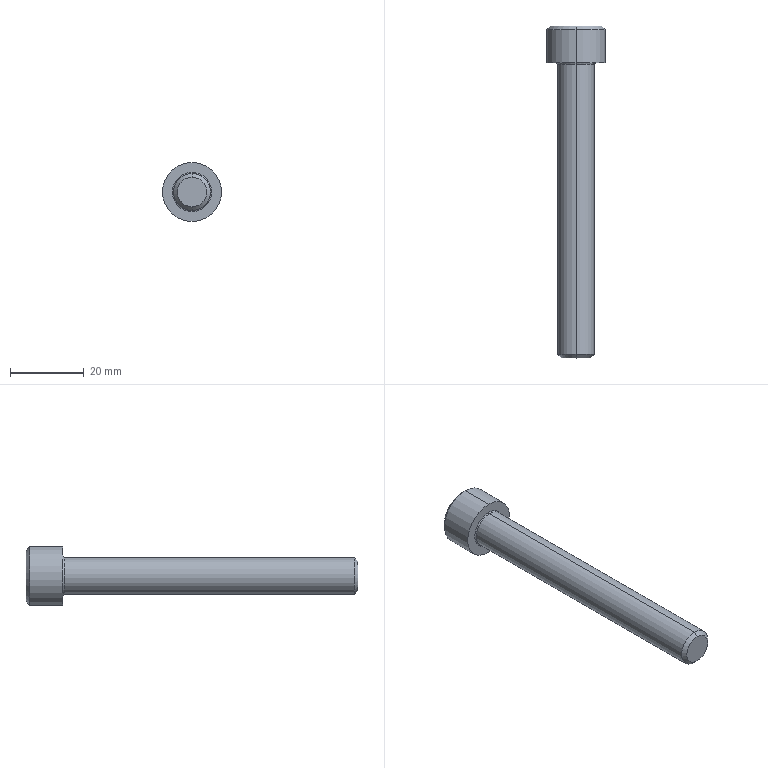Part | STEP file | 1 solid | 20 faces | box 16 x 90 x 16 mm | volume 7923 mm3 | plane 10 | cone 4 | cylinder 4 | spline 2 | commonest cylinder face diameters 10 x2 16 x2